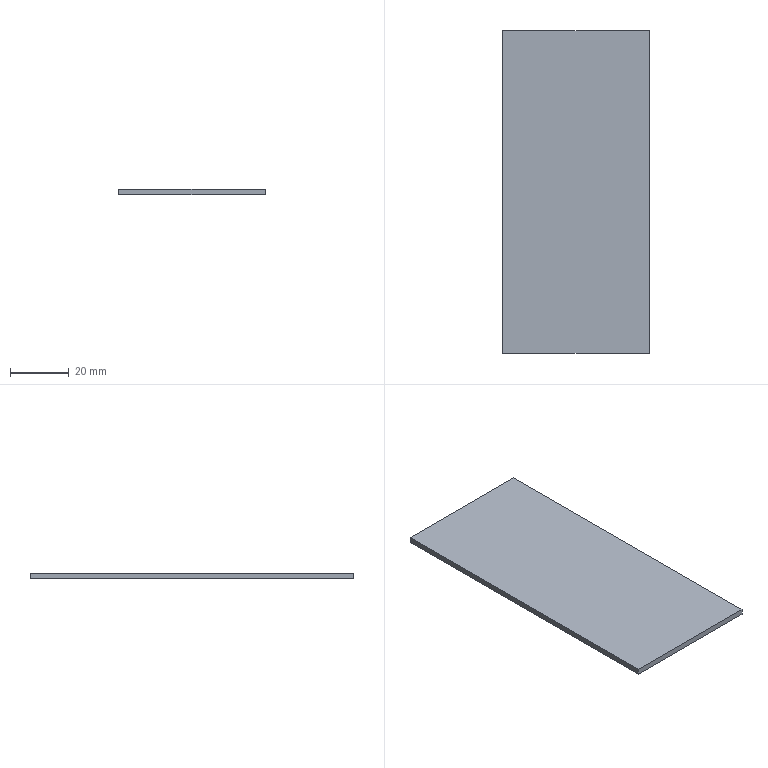Part | SolidWorks | features Extrusion 1 | 1 solid | 6 faces | box 50 x 110 x 2 mm | volume 11000 mm3 | plane 6
STEP:
#1=CARTESIAN_POINT('',(25.,-55.,-1.));
#2=VERTEX_POINT('',#1);
#3=CARTESIAN_POINT('',(25.,55.,-1.));
#4=VERTEX_POINT('',#3);
#5=CARTESIAN_POINT('',(25.,-55.,-1.));
#6=DIRECTION('',(0.,1.,0.));
#7=VECTOR('',#6,1000.);
#8=LINE('',#5,#7);
#9=EDGE_CURVE('',#2,#4,#8,.T.);
#10=ORIENTED_EDGE('',*,*,#9,.T.);
#11=CARTESIAN_POINT('',(25.,55.,1.));
#12=VERTEX_POINT('',#11);
#13=CARTESIAN_POINT('',(25.,55.,1.));
#14=DIRECTION('',(0.,0.,-1.));
#15=VECTOR('',#14,1000.);
#16=LINE('',#13,#15);
#17=EDGE_CURVE('',#12,#4,#16,.T.);
#18=ORIENTED_EDGE('',*,*,#17,.F.);
#19=CARTESIAN_POINT('',(25.,-55.,1.));
#20=VERTEX_POINT('',#19);
#21=CARTESIAN_POINT('',(25.,-55.,1.));
#22=DIRECTION('',(0.,1.,0.));
#23=VECTOR('',#22,1000.);
#24=LINE('',#21,#23);
#25=EDGE_CURVE('',#20,#12,#24,.T.);
#26=ORIENTED_EDGE('',*,*,#25,.F.);
#27=CARTESIAN_POINT('',(25.,-55.,1.));
#28=DIRECTION('',(0.,0.,-1.));
#29=VECTOR('',#28,1000.);
#30=LINE('',#27,#29);
#31=EDGE_CURVE('',#20,#2,#30,.T.);
#32=ORIENTED_EDGE('',*,*,#31,.T.);
#33=EDGE_LOOP('',(#10,#18,#26,#32));
#34=FACE_OUTER_BOUND('',#33,.T.);
#35=CARTESIAN_POINT('',(25.,-55.,1.));
#36=DIRECTION('',(-1.,0.,0.));
#37=DIRECTION('',(0.,0.,1.));
#38=AXIS2_PLACEMENT_3D('',#35,#36,#37);
#39=PLANE('',#38);
#40=ADVANCED_FACE('',(#34),#39,.F.);
#41=CARTESIAN_POINT('',(-25.,55.,-1.));
#42=VERTEX_POINT('',#41);
#43=CARTESIAN_POINT('',(-25.,55.,-1.));
#44=DIRECTION('',(-1.,0.,0.));
#45=VECTOR('',#44,1000.);
#46=LINE('',#43,#45);
#47=EDGE_CURVE('',#4,#42,#46,.T.);
#48=ORIENTED_EDGE('',*,*,#47,.T.);
#49=CARTESIAN_POINT('',(-25.,55.,1.));
#50=VERTEX_POINT('',#49);
#51=CARTESIAN_POINT('',(-25.,55.,1.));
#52=DIRECTION('',(0.,0.,-1.));
#53=VECTOR('',#52,1000.);
#54=LINE('',#51,#53);
#55=EDGE_CURVE('',#50,#42,#54,.T.);
#56=ORIENTED_EDGE('',*,*,#55,.F.);
#57=CARTESIAN_POINT('',(-25.,55.,1.));
#58=DIRECTION('',(-1.,0.,0.));
#59=VECTOR('',#58,1000.);
#60=LINE('',#57,#59);
#61=EDGE_CURVE('',#12,#50,#60,.T.);
#62=ORIENTED_EDGE('',*,*,#61,.F.);
#63=ORIENTED_EDGE('',*,*,#17,.T.);
#64=EDGE_LOOP('',(#48,#56,#62,#63));
#65=FACE_OUTER_BOUND('',#64,.T.);
#66=CARTESIAN_POINT('',(-25.,55.,1.));
#67=DIRECTION('',(0.,-1.,0.));
#68=DIRECTION('',(0.,0.,-1.));
#69=AXIS2_PLACEMENT_3D('',#66,#67,#68);
#70=PLANE('',#69);
#71=ADVANCED_FACE('',(#65),#70,.F.);
#72=CARTESIAN_POINT('',(-25.,-55.,-1.));
#73=VERTEX_POINT('',#72);
#74=CARTESIAN_POINT('',(-25.,-55.,-1.));
#75=DIRECTION('',(0.,-1.,0.));
#76=VECTOR('',#75,1000.);
#77=LINE('',#74,#76);
#78=EDGE_CURVE('',#42,#73,#77,.T.);
#79=ORIENTED_EDGE('',*,*,#78,.T.);
#80=CARTESIAN_POINT('',(-25.,-55.,1.));
#81=VERTEX_POINT('',#80);
#82=CARTESIAN_POINT('',(-25.,-55.,1.));
#83=DIRECTION('',(0.,0.,-1.));
#84=VECTOR('',#83,1000.);
#85=LINE('',#82,#84);
#86=EDGE_CURVE('',#81,#73,#85,.T.);
#87=ORIENTED_EDGE('',*,*,#86,.F.);
#88=CARTESIAN_POINT('',(-25.,-55.,1.));
#89=DIRECTION('',(0.,-1.,0.));
#90=VECTOR('',#89,1000.);
#91=LINE('',#88,#90);
#92=EDGE_CURVE('',#50,#81,#91,.T.);
#93=ORIENTED_EDGE('',*,*,#92,.F.);
#94=ORIENTED_EDGE('',*,*,#55,.T.);
#95=EDGE_LOOP('',(#79,#87,#93,#94));
#96=FACE_OUTER_BOUND('',#95,.T.);
#97=CARTESIAN_POINT('',(-25.,-55.,1.));
#98=DIRECTION('',(1.,0.,0.));
#99=DIRECTION('',(0.,0.,-1.));
#100=AXIS2_PLACEMENT_3D('',#97,#98,#99);
#101=PLANE('',#100);
#102=ADVANCED_FACE('',(#96),#101,.F.);
#103=CARTESIAN_POINT('',(-25.,-55.,-1.));
#104=DIRECTION('',(1.,0.,0.));
#105=VECTOR('',#104,1000.);
#106=LINE('',#103,#105);
#107=EDGE_CURVE('',#73,#2,#106,.T.);
#108=ORIENTED_EDGE('',*,*,#107,.T.);
#109=ORIENTED_EDGE('',*,*,#31,.F.);
#110=CARTESIAN_POINT('',(-25.,-55.,1.));
#111=DIRECTION('',(1.,0.,0.));
#112=VECTOR('',#111,1000.);
#113=LINE('',#110,#112);
#114=EDGE_CURVE('',#81,#20,#113,.T.);
#115=ORIENTED_EDGE('',*,*,#114,.F.);
#116=ORIENTED_EDGE('',*,*,#86,.T.);
#117=EDGE_LOOP('',(#108,#109,#115,#116));
#118=FACE_OUTER_BOUND('',#117,.T.);
#119=CARTESIAN_POINT('',(-25.,-55.,1.));
#120=DIRECTION('',(0.,1.,0.));
#121=DIRECTION('',(0.,0.,1.));
#122=AXIS2_PLACEMENT_3D('',#119,#120,#121);
#123=PLANE('',#122);
#124=ADVANCED_FACE('',(#118),#123,.F.);
#125=ORIENTED_EDGE('',*,*,#25,.T.);
#126=ORIENTED_EDGE('',*,*,#61,.T.);
#127=ORIENTED_EDGE('',*,*,#92,.T.);
#128=ORIENTED_EDGE('',*,*,#114,.T.);
#129=EDGE_LOOP('',(#125,#126,#127,#128));
#130=FACE_OUTER_BOUND('',#129,.T.);
#131=CARTESIAN_POINT('',(0.,0.,1.));
#132=DIRECTION('',(0.,0.,-1.));
#133=DIRECTION('',(-1.,0.,0.));
#134=AXIS2_PLACEMENT_3D('',#131,#132,#133);
#135=PLANE('',#134);
#136=ADVANCED_FACE('',(#130),#135,.F.);
#137=ORIENTED_EDGE('',*,*,#9,.F.);
#138=ORIENTED_EDGE('',*,*,#107,.F.);
#139=ORIENTED_EDGE('',*,*,#78,.F.);
#140=ORIENTED_EDGE('',*,*,#47,.F.);
#141=EDGE_LOOP('',(#137,#138,#139,#140));
#142=FACE_OUTER_BOUND('',#141,.T.);
#143=CARTESIAN_POINT('',(0.,0.,-1.));
#144=DIRECTION('',(0.,0.,-1.));
#145=DIRECTION('',(-1.,0.,0.));
#146=AXIS2_PLACEMENT_3D('',#143,#144,#145);
#147=PLANE('',#146);
#148=ADVANCED_FACE('',(#142),#147,.T.);
#149=CLOSED_SHELL('',(#40,#71,#102,#124,#136,#148));
#150=MANIFOLD_SOLID_BREP('',#149);
#151=CARTESIAN_POINT('',(0.,0.,0.));
#152=DIRECTION('',(0.,0.,1.));
#153=DIRECTION('',(1.,0.,0.));
#154=AXIS2_PLACEMENT_3D('',#151,#152,#153);
#155=(LENGTH_UNIT()NAMED_UNIT(*)SI_UNIT(.MILLI.,.METRE.));
#156=UNCERTAINTY_MEASURE_WITH_UNIT(LENGTH_MEASURE(0.00001),#155,'','');
#157=(NAMED_UNIT(*)PLANE_ANGLE_UNIT()SI_UNIT($,.RADIAN.));
#158=(NAMED_UNIT(*)SI_UNIT($,.STERADIAN.)SOLID_ANGLE_UNIT());
#159=(GEOMETRIC_REPRESENTATION_CONTEXT(3)GLOBAL_UNCERTAINTY_ASSIGNED_CONTEXT((#156))GLOBAL_UNIT_ASSIGNED_CONTEXT((#155,#157,#158))REPRESENTATION_CONTEXT('',''));
#160=ADVANCED_BREP_SHAPE_REPRESENTATION('',(#150,#154),#159);